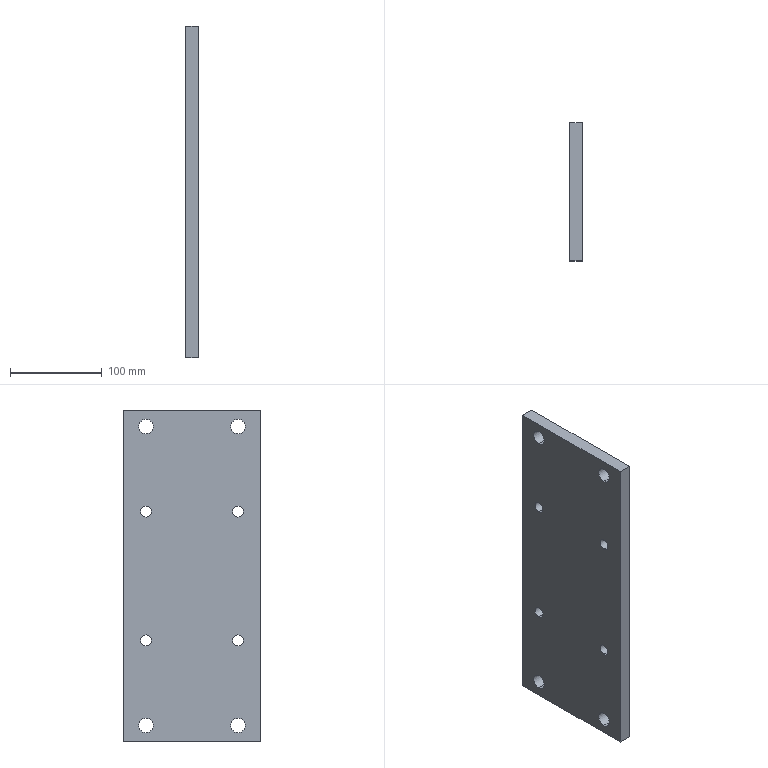Part | SolidWorks | features BaseBody 1 | 1 solid | 22 faces | box 14 x 150 x 360 mm | volume 738407 mm3 | cylinder 16 | plane 6 | commonest cylinder face diameters 12 x8 16 x8
STEP:
#1=CARTESIAN_POINT('',(14.,50.,-76.));
#2=VERTEX_POINT('',#1);
#3=CARTESIAN_POINT('',(14.,50.,-64.));
#4=VERTEX_POINT('',#3);
#5=CARTESIAN_POINT('',(14.,50.,-70.));
#6=DIRECTION('',(-1.,0.,0.));
#7=DIRECTION('',(0.,0.,1.));
#8=AXIS2_PLACEMENT_3D('',#5,#6,#7);
#9=CIRCLE('',#8,6.);
#10=EDGE_CURVE('',#2,#4,#9,.T.);
#11=ORIENTED_EDGE('',*,*,#10,.F.);
#12=CARTESIAN_POINT('',(0.,50.,-76.));
#13=VERTEX_POINT('',#12);
#14=CARTESIAN_POINT('',(14.,50.,-76.));
#15=DIRECTION('',(-1.,0.,0.));
#16=VECTOR('',#15,1000.);
#17=LINE('',#14,#16);
#18=EDGE_CURVE('',#2,#13,#17,.T.);
#19=ORIENTED_EDGE('',*,*,#18,.T.);
#20=CARTESIAN_POINT('',(0.,50.,-64.));
#21=VERTEX_POINT('',#20);
#22=CARTESIAN_POINT('',(0.,50.,-70.));
#23=DIRECTION('',(1.,0.,0.));
#24=DIRECTION('',(0.,0.,1.));
#25=AXIS2_PLACEMENT_3D('',#22,#23,#24);
#26=CIRCLE('',#25,6.);
#27=EDGE_CURVE('',#21,#13,#26,.T.);
#28=ORIENTED_EDGE('',*,*,#27,.F.);
#29=CARTESIAN_POINT('',(14.,50.,-64.));
#30=DIRECTION('',(-1.,0.,0.));
#31=VECTOR('',#30,1000.);
#32=LINE('',#29,#31);
#33=EDGE_CURVE('',#4,#21,#32,.T.);
#34=ORIENTED_EDGE('',*,*,#33,.F.);
#35=EDGE_LOOP('',(#11,#19,#28,#34));
#36=FACE_OUTER_BOUND('',#35,.T.);
#37=CARTESIAN_POINT('',(14.,50.,-70.));
#38=DIRECTION('',(-1.,0.,0.));
#39=DIRECTION('',(0.,0.,1.));
#40=AXIS2_PLACEMENT_3D('',#37,#38,#39);
#41=CYLINDRICAL_SURFACE('',#40,6.);
#42=ADVANCED_FACE('',(#36),#41,.F.);
#43=CARTESIAN_POINT('',(14.,-50.,64.));
#44=VERTEX_POINT('',#43);
#45=CARTESIAN_POINT('',(14.,-50.,76.));
#46=VERTEX_POINT('',#45);
#47=CARTESIAN_POINT('',(14.,-50.,70.));
#48=DIRECTION('',(-1.,0.,0.));
#49=DIRECTION('',(0.,0.,1.));
#50=AXIS2_PLACEMENT_3D('',#47,#48,#49);
#51=CIRCLE('',#50,6.);
#52=EDGE_CURVE('',#44,#46,#51,.T.);
#53=ORIENTED_EDGE('',*,*,#52,.F.);
#54=CARTESIAN_POINT('',(0.,-50.,64.));
#55=VERTEX_POINT('',#54);
#56=CARTESIAN_POINT('',(14.,-50.,64.));
#57=DIRECTION('',(-1.,0.,0.));
#58=VECTOR('',#57,1000.);
#59=LINE('',#56,#58);
#60=EDGE_CURVE('',#44,#55,#59,.T.);
#61=ORIENTED_EDGE('',*,*,#60,.T.);
#62=CARTESIAN_POINT('',(0.,-50.,76.));
#63=VERTEX_POINT('',#62);
#64=CARTESIAN_POINT('',(0.,-50.,70.));
#65=DIRECTION('',(1.,0.,0.));
#66=DIRECTION('',(0.,0.,1.));
#67=AXIS2_PLACEMENT_3D('',#64,#65,#66);
#68=CIRCLE('',#67,6.);
#69=EDGE_CURVE('',#63,#55,#68,.T.);
#70=ORIENTED_EDGE('',*,*,#69,.F.);
#71=CARTESIAN_POINT('',(14.,-50.,76.));
#72=DIRECTION('',(-1.,0.,0.));
#73=VECTOR('',#72,1000.);
#74=LINE('',#71,#73);
#75=EDGE_CURVE('',#46,#63,#74,.T.);
#76=ORIENTED_EDGE('',*,*,#75,.F.);
#77=EDGE_LOOP('',(#53,#61,#70,#76));
#78=FACE_OUTER_BOUND('',#77,.T.);
#79=CARTESIAN_POINT('',(14.,-50.,70.));
#80=DIRECTION('',(-1.,0.,0.));
#81=DIRECTION('',(0.,0.,1.));
#82=AXIS2_PLACEMENT_3D('',#79,#80,#81);
#83=CYLINDRICAL_SURFACE('',#82,6.);
#84=ADVANCED_FACE('',(#78),#83,.F.);
#85=CARTESIAN_POINT('',(14.,50.,64.));
#86=VERTEX_POINT('',#85);
#87=CARTESIAN_POINT('',(14.,50.,76.));
#88=VERTEX_POINT('',#87);
#89=CARTESIAN_POINT('',(14.,50.,70.));
#90=DIRECTION('',(-1.,0.,0.));
#91=DIRECTION('',(0.,0.,1.));
#92=AXIS2_PLACEMENT_3D('',#89,#90,#91);
#93=CIRCLE('',#92,6.);
#94=EDGE_CURVE('',#86,#88,#93,.T.);
#95=ORIENTED_EDGE('',*,*,#94,.F.);
#96=CARTESIAN_POINT('',(0.,50.,64.));
#97=VERTEX_POINT('',#96);
#98=CARTESIAN_POINT('',(14.,50.,64.));
#99=DIRECTION('',(-1.,0.,0.));
#100=VECTOR('',#99,1000.);
#101=LINE('',#98,#100);
#102=EDGE_CURVE('',#86,#97,#101,.T.);
#103=ORIENTED_EDGE('',*,*,#102,.T.);
#104=CARTESIAN_POINT('',(0.,50.,76.));
#105=VERTEX_POINT('',#104);
#106=CARTESIAN_POINT('',(0.,50.,70.));
#107=DIRECTION('',(1.,0.,0.));
#108=DIRECTION('',(0.,0.,1.));
#109=AXIS2_PLACEMENT_3D('',#106,#107,#108);
#110=CIRCLE('',#109,6.);
#111=EDGE_CURVE('',#105,#97,#110,.T.);
#112=ORIENTED_EDGE('',*,*,#111,.F.);
#113=CARTESIAN_POINT('',(14.,50.,76.));
#114=DIRECTION('',(-1.,0.,0.));
#115=VECTOR('',#114,1000.);
#116=LINE('',#113,#115);
#117=EDGE_CURVE('',#88,#105,#116,.T.);
#118=ORIENTED_EDGE('',*,*,#117,.F.);
#119=EDGE_LOOP('',(#95,#103,#112,#118));
#120=FACE_OUTER_BOUND('',#119,.T.);
#121=CARTESIAN_POINT('',(14.,50.,70.));
#122=DIRECTION('',(-1.,0.,0.));
#123=DIRECTION('',(0.,0.,1.));
#124=AXIS2_PLACEMENT_3D('',#121,#122,#123);
#125=CYLINDRICAL_SURFACE('',#124,6.);
#126=ADVANCED_FACE('',(#120),#125,.F.);
#127=CARTESIAN_POINT('',(14.,-50.,-76.));
#128=VERTEX_POINT('',#127);
#129=CARTESIAN_POINT('',(14.,-50.,-64.));
#130=VERTEX_POINT('',#129);
#131=CARTESIAN_POINT('',(14.,-50.,-70.));
#132=DIRECTION('',(-1.,0.,0.));
#133=DIRECTION('',(0.,0.,1.));
#134=AXIS2_PLACEMENT_3D('',#131,#132,#133);
#135=CIRCLE('',#134,6.);
#136=EDGE_CURVE('',#128,#130,#135,.T.);
#137=ORIENTED_EDGE('',*,*,#136,.F.);
#138=CARTESIAN_POINT('',(0.,-50.,-76.));
#139=VERTEX_POINT('',#138);
#140=CARTESIAN_POINT('',(14.,-50.,-76.));
#141=DIRECTION('',(-1.,0.,0.));
#142=VECTOR('',#141,1000.);
#143=LINE('',#140,#142);
#144=EDGE_CURVE('',#128,#139,#143,.T.);
#145=ORIENTED_EDGE('',*,*,#144,.T.);
#146=CARTESIAN_POINT('',(0.,-50.,-64.));
#147=VERTEX_POINT('',#146);
#148=CARTESIAN_POINT('',(0.,-50.,-70.));
#149=DIRECTION('',(1.,0.,0.));
#150=DIRECTION('',(0.,0.,1.));
#151=AXIS2_PLACEMENT_3D('',#148,#149,#150);
#152=CIRCLE('',#151,6.);
#153=EDGE_CURVE('',#147,#139,#152,.T.);
#154=ORIENTED_EDGE('',*,*,#153,.F.);
#155=CARTESIAN_POINT('',(14.,-50.,-64.));
#156=DIRECTION('',(-1.,0.,0.));
#157=VECTOR('',#156,1000.);
#158=LINE('',#155,#157);
#159=EDGE_CURVE('',#130,#147,#158,.T.);
#160=ORIENTED_EDGE('',*,*,#159,.F.);
#161=EDGE_LOOP('',(#137,#145,#154,#160));
#162=FACE_OUTER_BOUND('',#161,.T.);
#163=CARTESIAN_POINT('',(14.,-50.,-70.));
#164=DIRECTION('',(-1.,0.,0.));
#165=DIRECTION('',(0.,0.,1.));
#166=AXIS2_PLACEMENT_3D('',#163,#164,#165);
#167=CYLINDRICAL_SURFACE('',#166,6.);
#168=ADVANCED_FACE('',(#162),#167,.F.);
#169=CARTESIAN_POINT('',(14.,50.,-170.5));
#170=VERTEX_POINT('',#169);
#171=CARTESIAN_POINT('',(14.,50.,-154.5));
#172=VERTEX_POINT('',#171);
#173=CARTESIAN_POINT('',(14.,50.,-162.5));
#174=DIRECTION('',(-1.,0.,0.));
#175=DIRECTION('',(0.,0.,1.));
#176=AXIS2_PLACEMENT_3D('',#173,#174,#175);
#177=CIRCLE('',#176,8.);
#178=EDGE_CURVE('',#170,#172,#177,.T.);
#179=ORIENTED_EDGE('',*,*,#178,.F.);
#180=CARTESIAN_POINT('',(0.,50.,-170.5));
#181=VERTEX_POINT('',#180);
#182=CARTESIAN_POINT('',(14.,50.,-170.5));
#183=DIRECTION('',(-1.,0.,0.));
#184=VECTOR('',#183,1000.);
#185=LINE('',#182,#184);
#186=EDGE_CURVE('',#170,#181,#185,.T.);
#187=ORIENTED_EDGE('',*,*,#186,.T.);
#188=CARTESIAN_POINT('',(0.,50.,-154.5));
#189=VERTEX_POINT('',#188);
#190=CARTESIAN_POINT('',(0.,50.,-162.5));
#191=DIRECTION('',(1.,0.,0.));
#192=DIRECTION('',(0.,0.,1.));
#193=AXIS2_PLACEMENT_3D('',#190,#191,#192);
#194=CIRCLE('',#193,8.);
#195=EDGE_CURVE('',#189,#181,#194,.T.);
#196=ORIENTED_EDGE('',*,*,#195,.F.);
#197=CARTESIAN_POINT('',(14.,50.,-154.5));
#198=DIRECTION('',(-1.,0.,0.));
#199=VECTOR('',#198,1000.);
#200=LINE('',#197,#199);
#201=EDGE_CURVE('',#172,#189,#200,.T.);
#202=ORIENTED_EDGE('',*,*,#201,.F.);
#203=EDGE_LOOP('',(#179,#187,#196,#202));
#204=FACE_OUTER_BOUND('',#203,.T.);
#205=CARTESIAN_POINT('',(14.,50.,-162.5));
#206=DIRECTION('',(-1.,0.,0.));
#207=DIRECTION('',(0.,0.,1.));
#208=AXIS2_PLACEMENT_3D('',#205,#206,#207);
#209=CYLINDRICAL_SURFACE('',#208,8.);
#210=ADVANCED_FACE('',(#204),#209,.F.);
#211=CARTESIAN_POINT('',(14.,-50.,-170.5));
#212=VERTEX_POINT('',#211);
#213=CARTESIAN_POINT('',(14.,-50.,-154.5));
#214=VERTEX_POINT('',#213);
#215=CARTESIAN_POINT('',(14.,-50.,-162.5));
#216=DIRECTION('',(-1.,0.,0.));
#217=DIRECTION('',(0.,0.,1.));
#218=AXIS2_PLACEMENT_3D('',#215,#216,#217);
#219=CIRCLE('',#218,8.);
#220=EDGE_CURVE('',#212,#214,#219,.T.);
#221=ORIENTED_EDGE('',*,*,#220,.F.);
#222=CARTESIAN_POINT('',(0.,-50.,-170.5));
#223=VERTEX_POINT('',#222);
#224=CARTESIAN_POINT('',(14.,-50.,-170.5));
#225=DIRECTION('',(-1.,0.,0.));
#226=VECTOR('',#225,1000.);
#227=LINE('',#224,#226);
#228=EDGE_CURVE('',#212,#223,#227,.T.);
#229=ORIENTED_EDGE('',*,*,#228,.T.);
#230=CARTESIAN_POINT('',(0.,-50.,-154.5));
#231=VERTEX_POINT('',#230);
#232=CARTESIAN_POINT('',(0.,-50.,-162.5));
#233=DIRECTION('',(1.,0.,0.));
#234=DIRECTION('',(0.,0.,1.));
#235=AXIS2_PLACEMENT_3D('',#232,#233,#234);
#236=CIRCLE('',#235,8.);
#237=EDGE_CURVE('',#231,#223,#236,.T.);
#238=ORIENTED_EDGE('',*,*,#237,.F.);
#239=CARTESIAN_POINT('',(14.,-50.,-154.5));
#240=DIRECTION('',(-1.,0.,0.));
#241=VECTOR('',#240,1000.);
#242=LINE('',#239,#241);
#243=EDGE_CURVE('',#214,#231,#242,.T.);
#244=ORIENTED_EDGE('',*,*,#243,.F.);
#245=EDGE_LOOP('',(#221,#229,#238,#244));
#246=FACE_OUTER_BOUND('',#245,.T.);
#247=CARTESIAN_POINT('',(14.,-50.,-162.5));
#248=DIRECTION('',(-1.,0.,0.));
#249=DIRECTION('',(0.,0.,1.));
#250=AXIS2_PLACEMENT_3D('',#247,#248,#249);
#251=CYLINDRICAL_SURFACE('',#250,8.);
#252=ADVANCED_FACE('',(#246),#251,.F.);
#253=CARTESIAN_POINT('',(14.,-50.,154.5));
#254=VERTEX_POINT('',#253);
#255=CARTESIAN_POINT('',(14.,-50.,170.5));
#256=VERTEX_POINT('',#255);
#257=CARTESIAN_POINT('',(14.,-50.,162.5));
#258=DIRECTION('',(-1.,0.,0.));
#259=DIRECTION('',(0.,0.,1.));
#260=AXIS2_PLACEMENT_3D('',#257,#258,#259);
#261=CIRCLE('',#260,8.);
#262=EDGE_CURVE('',#254,#256,#261,.T.);
#263=ORIENTED_EDGE('',*,*,#262,.F.);
#264=CARTESIAN_POINT('',(0.,-50.,154.5));
#265=VERTEX_POINT('',#264);
#266=CARTESIAN_POINT('',(14.,-50.,154.5));
#267=DIRECTION('',(-1.,0.,0.));
#268=VECTOR('',#267,1000.);
#269=LINE('',#266,#268);
#270=EDGE_CURVE('',#254,#265,#269,.T.);
#271=ORIENTED_EDGE('',*,*,#270,.T.);
#272=CARTESIAN_POINT('',(0.,-50.,170.5));
#273=VERTEX_POINT('',#272);
#274=CARTESIAN_POINT('',(0.,-50.,162.5));
#275=DIRECTION('',(1.,0.,0.));
#276=DIRECTION('',(0.,0.,1.));
#277=AXIS2_PLACEMENT_3D('',#274,#275,#276);
#278=CIRCLE('',#277,8.);
#279=EDGE_CURVE('',#273,#265,#278,.T.);
#280=ORIENTED_EDGE('',*,*,#279,.F.);
#281=CARTESIAN_POINT('',(14.,-50.,170.5));
#282=DIRECTION('',(-1.,0.,0.));
#283=VECTOR('',#282,1000.);
#284=LINE('',#281,#283);
#285=EDGE_CURVE('',#256,#273,#284,.T.);
#286=ORIENTED_EDGE('',*,*,#285,.F.);
#287=EDGE_LOOP('',(#263,#271,#280,#286));
#288=FACE_OUTER_BOUND('',#287,.T.);
#289=CARTESIAN_POINT('',(14.,-50.,162.5));
#290=DIRECTION('',(-1.,0.,0.));
#291=DIRECTION('',(0.,0.,1.));
#292=AXIS2_PLACEMENT_3D('',#289,#290,#291);
#293=CYLINDRICAL_SURFACE('',#292,8.);
#294=ADVANCED_FACE('',(#288),#293,.F.);
#295=CARTESIAN_POINT('',(14.,50.,154.5));
#296=VERTEX_POINT('',#295);
#297=CARTESIAN_POINT('',(14.,50.,170.5));
#298=VERTEX_POINT('',#297);
#299=CARTESIAN_POINT('',(14.,50.,162.5));
#300=DIRECTION('',(-1.,0.,0.));
#301=DIRECTION('',(0.,0.,1.));
#302=AXIS2_PLACEMENT_3D('',#299,#300,#301);
#303=CIRCLE('',#302,8.);
#304=EDGE_CURVE('',#296,#298,#303,.T.);
#305=ORIENTED_EDGE('',*,*,#304,.F.);
#306=CARTESIAN_POINT('',(0.,50.,154.5));
#307=VERTEX_POINT('',#306);
#308=CARTESIAN_POINT('',(14.,50.,154.5));
#309=DIRECTION('',(-1.,0.,0.));
#310=VECTOR('',#309,1000.);
#311=LINE('',#308,#310);
#312=EDGE_CURVE('',#296,#307,#311,.T.);
#313=ORIENTED_EDGE('',*,*,#312,.T.);
#314=CARTESIAN_POINT('',(0.,50.,170.5));
#315=VERTEX_POINT('',#314);
#316=CARTESIAN_POINT('',(0.,50.,162.5));
#317=DIRECTION('',(1.,0.,0.));
#318=DIRECTION('',(0.,0.,1.));
#319=AXIS2_PLACEMENT_3D('',#316,#317,#318);
#320=CIRCLE('',#319,8.);
#321=EDGE_CURVE('',#315,#307,#320,.T.);
#322=ORIENTED_EDGE('',*,*,#321,.F.);
#323=CARTESIAN_POINT('',(14.,50.,170.5));
#324=DIRECTION('',(-1.,0.,0.));
#325=VECTOR('',#324,1000.);
#326=LINE('',#323,#325);
#327=EDGE_CURVE('',#298,#315,#326,.T.);
#328=ORIENTED_EDGE('',*,*,#327,.F.);
#329=EDGE_LOOP('',(#305,#313,#322,#328));
#330=FACE_OUTER_BOUND('',#329,.T.);
#331=CARTESIAN_POINT('',(14.,50.,162.5));
#332=DIRECTION('',(-1.,0.,0.));
#333=DIRECTION('',(0.,0.,1.));
#334=AXIS2_PLACEMENT_3D('',#331,#332,#333);
#335=CYLINDRICAL_SURFACE('',#334,8.);
#336=ADVANCED_FACE('',(#330),#335,.F.);
#337=ORIENTED_EDGE('',*,*,#27,.T.);
#338=CARTESIAN_POINT('',(0.,50.,-70.));
#339=DIRECTION('',(1.,0.,0.));
#340=DIRECTION('',(0.,0.,1.));
#341=AXIS2_PLACEMENT_3D('',#338,#339,#340);
#342=CIRCLE('',#341,6.);
#343=EDGE_CURVE('',#13,#21,#342,.T.);
#344=ORIENTED_EDGE('',*,*,#343,.T.);
#345=EDGE_LOOP('',(#337,#344));
#346=FACE_BOUND('',#345,.T.);
#347=ORIENTED_EDGE('',*,*,#69,.T.);
#348=CARTESIAN_POINT('',(0.,-50.,70.));
#349=DIRECTION('',(1.,0.,0.));
#350=DIRECTION('',(0.,0.,1.));
#351=AXIS2_PLACEMENT_3D('',#348,#349,#350);
#352=CIRCLE('',#351,6.);
#353=EDGE_CURVE('',#55,#63,#352,.T.);
#354=ORIENTED_EDGE('',*,*,#353,.T.);
#355=EDGE_LOOP('',(#347,#354));
#356=FACE_BOUND('',#355,.T.);
#357=CARTESIAN_POINT('',(0.,-75.,180.));
#358=VERTEX_POINT('',#357);
#359=CARTESIAN_POINT('',(0.,75.,180.));
#360=VERTEX_POINT('',#359);
#361=CARTESIAN_POINT('',(0.,0.,180.));
#362=DIRECTION('',(0.,1.,0.));
#363=VECTOR('',#362,1000.);
#364=LINE('',#361,#363);
#365=EDGE_CURVE('',#358,#360,#364,.T.);
#366=ORIENTED_EDGE('',*,*,#365,.T.);
#367=CARTESIAN_POINT('',(0.,75.,-180.));
#368=VERTEX_POINT('',#367);
#369=CARTESIAN_POINT('',(0.,75.,0.));
#370=DIRECTION('',(0.,0.,-1.));
#371=VECTOR('',#370,1000.);
#372=LINE('',#369,#371);
#373=EDGE_CURVE('',#360,#368,#372,.T.);
#374=ORIENTED_EDGE('',*,*,#373,.T.);
#375=CARTESIAN_POINT('',(0.,-75.,-180.));
#376=VERTEX_POINT('',#375);
#377=CARTESIAN_POINT('',(0.,0.,-180.));
#378=DIRECTION('',(0.,-1.,0.));
#379=VECTOR('',#378,1000.);
#380=LINE('',#377,#379);
#381=EDGE_CURVE('',#368,#376,#380,.T.);
#382=ORIENTED_EDGE('',*,*,#381,.T.);
#383=CARTESIAN_POINT('',(0.,-75.,0.));
#384=DIRECTION('',(0.,0.,1.));
#385=VECTOR('',#384,1000.);
#386=LINE('',#383,#385);
#387=EDGE_CURVE('',#376,#358,#386,.T.);
#388=ORIENTED_EDGE('',*,*,#387,.T.);
#389=EDGE_LOOP('',(#366,#374,#382,#388));
#390=FACE_OUTER_BOUND('',#389,.T.);
#391=ORIENTED_EDGE('',*,*,#111,.T.);
#392=CARTESIAN_POINT('',(0.,50.,70.));
#393=DIRECTION('',(1.,0.,0.));
#394=DIRECTION('',(0.,0.,1.));
#395=AXIS2_PLACEMENT_3D('',#392,#393,#394);
#396=CIRCLE('',#395,6.);
#397=EDGE_CURVE('',#97,#105,#396,.T.);
#398=ORIENTED_EDGE('',*,*,#397,.T.);
#399=EDGE_LOOP('',(#391,#398));
#400=FACE_BOUND('',#399,.T.);
#401=ORIENTED_EDGE('',*,*,#153,.T.);
#402=CARTESIAN_POINT('',(0.,-50.,-70.));
#403=DIRECTION('',(1.,0.,0.));
#404=DIRECTION('',(0.,0.,1.));
#405=AXIS2_PLACEMENT_3D('',#402,#403,#404);
#406=CIRCLE('',#405,6.);
#407=EDGE_CURVE('',#139,#147,#406,.T.);
#408=ORIENTED_EDGE('',*,*,#407,.T.);
#409=EDGE_LOOP('',(#401,#408));
#410=FACE_BOUND('',#409,.T.);
#411=ORIENTED_EDGE('',*,*,#195,.T.);
#412=CARTESIAN_POINT('',(0.,50.,-162.5));
#413=DIRECTION('',(1.,0.,0.));
#414=DIRECTION('',(0.,0.,1.));
#415=AXIS2_PLACEMENT_3D('',#412,#413,#414);
#416=CIRCLE('',#415,8.);
#417=EDGE_CURVE('',#181,#189,#416,.T.);
#418=ORIENTED_EDGE('',*,*,#417,.T.);
#419=EDGE_LOOP('',(#411,#418));
#420=FACE_BOUND('',#419,.T.);
#421=ORIENTED_EDGE('',*,*,#237,.T.);
#422=CARTESIAN_POINT('',(0.,-50.,-162.5));
#423=DIRECTION('',(1.,0.,0.));
#424=DIRECTION('',(0.,0.,1.));
#425=AXIS2_PLACEMENT_3D('',#422,#423,#424);
#426=CIRCLE('',#425,8.);
#427=EDGE_CURVE('',#223,#231,#426,.T.);
#428=ORIENTED_EDGE('',*,*,#427,.T.);
#429=EDGE_LOOP('',(#421,#428));
#430=FACE_BOUND('',#429,.T.);
#431=ORIENTED_EDGE('',*,*,#279,.T.);
#432=CARTESIAN_POINT('',(0.,-50.,162.5));
#433=DIRECTION('',(1.,0.,0.));
#434=DIRECTION('',(0.,0.,1.));
#435=AXIS2_PLACEMENT_3D('',#432,#433,#434);
#436=CIRCLE('',#435,8.);
#437=EDGE_CURVE('',#265,#273,#436,.T.);
#438=ORIENTED_EDGE('',*,*,#437,.T.);
#439=EDGE_LOOP('',(#431,#438));
#440=FACE_BOUND('',#439,.T.);
#441=ORIENTED_EDGE('',*,*,#321,.T.);
#442=CARTESIAN_POINT('',(0.,50.,162.5));
#443=DIRECTION('',(1.,0.,0.));
#444=DIRECTION('',(0.,0.,1.));
#445=AXIS2_PLACEMENT_3D('',#442,#443,#444);
#446=CIRCLE('',#445,8.);
#447=EDGE_CURVE('',#307,#315,#446,.T.);
#448=ORIENTED_EDGE('',*,*,#447,.T.);
#449=EDGE_LOOP('',(#441,#448));
#450=FACE_BOUND('',#449,.T.);
#451=CARTESIAN_POINT('',(0.,0.,0.));
#452=DIRECTION('',(-1.,0.,0.));
#453=DIRECTION('',(0.,0.,1.));
#454=AXIS2_PLACEMENT_3D('',#451,#452,#453);
#455=PLANE('',#454);
#456=ADVANCED_FACE('',(#346,#356,#390,#400,#410,#420,#430,#440,#450),#455,.T.);
#457=ORIENTED_EDGE('',*,*,#18,.F.);
#458=CARTESIAN_POINT('',(14.,50.,-70.));
#459=DIRECTION('',(-1.,0.,0.));
#460=DIRECTION('',(0.,0.,1.));
#461=AXIS2_PLACEMENT_3D('',#458,#459,#460);
#462=CIRCLE('',#461,6.);
#463=EDGE_CURVE('',#4,#2,#462,.T.);
#464=ORIENTED_EDGE('',*,*,#463,.F.);
#465=ORIENTED_EDGE('',*,*,#33,.T.);
#466=ORIENTED_EDGE('',*,*,#343,.F.);
#467=EDGE_LOOP('',(#457,#464,#465,#466));
#468=FACE_OUTER_BOUND('',#467,.T.);
#469=CARTESIAN_POINT('',(14.,50.,-70.));
#470=DIRECTION('',(-1.,0.,0.));
#471=DIRECTION('',(0.,0.,1.));
#472=AXIS2_PLACEMENT_3D('',#469,#470,#471);
#473=CYLINDRICAL_SURFACE('',#472,6.);
#474=ADVANCED_FACE('',(#468),#473,.F.);
#475=ORIENTED_EDGE('',*,*,#60,.F.);
#476=CARTESIAN_POINT('',(14.,-50.,70.));
#477=DIRECTION('',(-1.,0.,0.));
#478=DIRECTION('',(0.,0.,1.));
#479=AXIS2_PLACEMENT_3D('',#476,#477,#478);
#480=CIRCLE('',#479,6.);
#481=EDGE_CURVE('',#46,#44,#480,.T.);
#482=ORIENTED_EDGE('',*,*,#481,.F.);
#483=ORIENTED_EDGE('',*,*,#75,.T.);
#484=ORIENTED_EDGE('',*,*,#353,.F.);
#485=EDGE_LOOP('',(#475,#482,#483,#484));
#486=FACE_OUTER_BOUND('',#485,.T.);
#487=CARTESIAN_POINT('',(14.,-50.,70.));
#488=DIRECTION('',(-1.,0.,0.));
#489=DIRECTION('',(0.,0.,1.));
#490=AXIS2_PLACEMENT_3D('',#487,#488,#489);
#491=CYLINDRICAL_SURFACE('',#490,6.);
#492=ADVANCED_FACE('',(#486),#491,.F.);
#493=CARTESIAN_POINT('',(14.,75.,180.));
#494=VERTEX_POINT('',#493);
#495=CARTESIAN_POINT('',(14.,75.,180.));
#496=DIRECTION('',(-1.,0.,0.));
#497=VECTOR('',#496,1000.);
#498=LINE('',#495,#497);
#499=EDGE_CURVE('',#494,#360,#498,.T.);
#500=ORIENTED_EDGE('',*,*,#499,.F.);
#501=CARTESIAN_POINT('',(14.,75.,-180.));
#502=VERTEX_POINT('',#501);
#503=CARTESIAN_POINT('',(14.,75.,180.));
#504=DIRECTION('',(0.,0.,1.));
#505=VECTOR('',#504,1000.);
#506=LINE('',#503,#505);
#507=EDGE_CURVE('',#502,#494,#506,.T.);
#508=ORIENTED_EDGE('',*,*,#507,.F.);
#509=CARTESIAN_POINT('',(14.,75.,-180.));
#510=DIRECTION('',(1.,0.,0.));
#511=VECTOR('',#510,1000.);
#512=LINE('',#509,#511);
#513=EDGE_CURVE('',#368,#502,#512,.T.);
#514=ORIENTED_EDGE('',*,*,#513,.F.);
#515=ORIENTED_EDGE('',*,*,#373,.F.);
#516=EDGE_LOOP('',(#500,#508,#514,#515));
#517=FACE_OUTER_BOUND('',#516,.T.);
#518=CARTESIAN_POINT('',(14.,75.,180.));
#519=DIRECTION('',(0.,-1.,0.));
#520=DIRECTION('',(0.,0.,-1.));
#521=AXIS2_PLACEMENT_3D('',#518,#519,#520);
#522=PLANE('',#521);
#523=ADVANCED_FACE('',(#517),#522,.F.);
#524=CARTESIAN_POINT('',(14.,-75.,180.));
#525=VERTEX_POINT('',#524);
#526=CARTESIAN_POINT('',(14.,-75.,180.));
#527=DIRECTION('',(-1.,0.,0.));
#528=VECTOR('',#527,1000.);
#529=LINE('',#526,#528);
#530=EDGE_CURVE('',#525,#358,#529,.T.);
#531=ORIENTED_EDGE('',*,*,#530,.F.);
#532=CARTESIAN_POINT('',(14.,-75.,180.));
#533=DIRECTION('',(0.,-1.,0.));
#534=VECTOR('',#533,1000.);
#535=LINE('',#532,#534);
#536=EDGE_CURVE('',#494,#525,#535,.T.);
#537=ORIENTED_EDGE('',*,*,#536,.F.);
#538=ORIENTED_EDGE('',*,*,#499,.T.);
#539=ORIENTED_EDGE('',*,*,#365,.F.);
#540=EDGE_LOOP('',(#531,#537,#538,#539));
#541=FACE_OUTER_BOUND('',#540,.T.);
#542=CARTESIAN_POINT('',(14.,-75.,180.));
#543=DIRECTION('',(0.,0.,-1.));
#544=DIRECTION('',(-1.,0.,0.));
#545=AXIS2_PLACEMENT_3D('',#542,#543,#544);
#546=PLANE('',#545);
#547=ADVANCED_FACE('',(#541),#546,.F.);
#548=CARTESIAN_POINT('',(14.,-75.,-180.));
#549=VERTEX_POINT('',#548);
#550=CARTESIAN_POINT('',(14.,-75.,-180.));
#551=DIRECTION('',(-1.,0.,0.));
#552=VECTOR('',#551,1000.);
#553=LINE('',#550,#552);
#554=EDGE_CURVE('',#549,#376,#553,.T.);
#555=ORIENTED_EDGE('',*,*,#554,.F.);
#556=CARTESIAN_POINT('',(14.,-75.,180.));
#557=DIRECTION('',(0.,0.,-1.));
#558=VECTOR('',#557,1000.);
#559=LINE('',#556,#558);
#560=EDGE_CURVE('',#525,#549,#559,.T.);
#561=ORIENTED_EDGE('',*,*,#560,.F.);
#562=ORIENTED_EDGE('',*,*,#530,.T.);
#563=ORIENTED_EDGE('',*,*,#387,.F.);
#564=EDGE_LOOP('',(#555,#561,#562,#563));
#565=FACE_OUTER_BOUND('',#564,.T.);
#566=CARTESIAN_POINT('',(14.,-75.,180.));
#567=DIRECTION('',(0.,1.,0.));
#568=DIRECTION('',(0.,0.,1.));
#569=AXIS2_PLACEMENT_3D('',#566,#567,#568);
#570=PLANE('',#569);
#571=ADVANCED_FACE('',(#565),#570,.F.);
#572=ORIENTED_EDGE('',*,*,#513,.T.);
#573=CARTESIAN_POINT('',(14.,-75.,-180.));
#574=DIRECTION('',(0.,1.,0.));
#575=VECTOR('',#574,1000.);
#576=LINE('',#573,#575);
#577=EDGE_CURVE('',#549,#502,#576,.T.);
#578=ORIENTED_EDGE('',*,*,#577,.F.);
#579=ORIENTED_EDGE('',*,*,#554,.T.);
#580=ORIENTED_EDGE('',*,*,#381,.F.);
#581=EDGE_LOOP('',(#572,#578,#579,#580));
#582=FACE_OUTER_BOUND('',#581,.T.);
#583=CARTESIAN_POINT('',(14.,-75.,-180.));
#584=DIRECTION('',(0.,0.,1.));
#585=DIRECTION('',(1.,0.,0.));
#586=AXIS2_PLACEMENT_3D('',#583,#584,#585);
#587=PLANE('',#586);
#588=ADVANCED_FACE('',(#582),#587,.F.);
#589=ORIENTED_EDGE('',*,*,#102,.F.);
#590=CARTESIAN_POINT('',(14.,50.,70.));
#591=DIRECTION('',(-1.,0.,0.));
#592=DIRECTION('',(0.,0.,1.));
#593=AXIS2_PLACEMENT_3D('',#590,#591,#592);
#594=CIRCLE('',#593,6.);
#595=EDGE_CURVE('',#88,#86,#594,.T.);
#596=ORIENTED_EDGE('',*,*,#595,.F.);
#597=ORIENTED_EDGE('',*,*,#117,.T.);
#598=ORIENTED_EDGE('',*,*,#397,.F.);
#599=EDGE_LOOP('',(#589,#596,#597,#598));
#600=FACE_OUTER_BOUND('',#599,.T.);
#601=CARTESIAN_POINT('',(14.,50.,70.));
#602=DIRECTION('',(-1.,0.,0.));
#603=DIRECTION('',(0.,0.,1.));
#604=AXIS2_PLACEMENT_3D('',#601,#602,#603);
#605=CYLINDRICAL_SURFACE('',#604,6.);
#606=ADVANCED_FACE('',(#600),#605,.F.);
#607=ORIENTED_EDGE('',*,*,#144,.F.);
#608=CARTESIAN_POINT('',(14.,-50.,-70.));
#609=DIRECTION('',(-1.,0.,0.));
#610=DIRECTION('',(0.,0.,1.));
#611=AXIS2_PLACEMENT_3D('',#608,#609,#610);
#612=CIRCLE('',#611,6.);
#613=EDGE_CURVE('',#130,#128,#612,.T.);
#614=ORIENTED_EDGE('',*,*,#613,.F.);
#615=ORIENTED_EDGE('',*,*,#159,.T.);
#616=ORIENTED_EDGE('',*,*,#407,.F.);
#617=EDGE_LOOP('',(#607,#614,#615,#616));
#618=FACE_OUTER_BOUND('',#617,.T.);
#619=CARTESIAN_POINT('',(14.,-50.,-70.));
#620=DIRECTION('',(-1.,0.,0.));
#621=DIRECTION('',(0.,0.,1.));
#622=AXIS2_PLACEMENT_3D('',#619,#620,#621);
#623=CYLINDRICAL_SURFACE('',#622,6.);
#624=ADVANCED_FACE('',(#618),#623,.F.);
#625=ORIENTED_EDGE('',*,*,#186,.F.);
#626=CARTESIAN_POINT('',(14.,50.,-162.5));
#627=DIRECTION('',(-1.,0.,0.));
#628=DIRECTION('',(0.,0.,1.));
#629=AXIS2_PLACEMENT_3D('',#626,#627,#628);
#630=CIRCLE('',#629,8.);
#631=EDGE_CURVE('',#172,#170,#630,.T.);
#632=ORIENTED_EDGE('',*,*,#631,.F.);
#633=ORIENTED_EDGE('',*,*,#201,.T.);
#634=ORIENTED_EDGE('',*,*,#417,.F.);
#635=EDGE_LOOP('',(#625,#632,#633,#634));
#636=FACE_OUTER_BOUND('',#635,.T.);
#637=CARTESIAN_POINT('',(14.,50.,-162.5));
#638=DIRECTION('',(-1.,0.,0.));
#639=DIRECTION('',(0.,0.,1.));
#640=AXIS2_PLACEMENT_3D('',#637,#638,#639);
#641=CYLINDRICAL_SURFACE('',#640,8.);
#642=ADVANCED_FACE('',(#636),#641,.F.);
#643=ORIENTED_EDGE('',*,*,#228,.F.);
#644=CARTESIAN_POINT('',(14.,-50.,-162.5));
#645=DIRECTION('',(-1.,0.,0.));
#646=DIRECTION('',(0.,0.,1.));
#647=AXIS2_PLACEMENT_3D('',#644,#645,#646);
#648=CIRCLE('',#647,8.);
#649=EDGE_CURVE('',#214,#212,#648,.T.);
#650=ORIENTED_EDGE('',*,*,#649,.F.);
#651=ORIENTED_EDGE('',*,*,#243,.T.);
#652=ORIENTED_EDGE('',*,*,#427,.F.);
#653=EDGE_LOOP('',(#643,#650,#651,#652));
#654=FACE_OUTER_BOUND('',#653,.T.);
#655=CARTESIAN_POINT('',(14.,-50.,-162.5));
#656=DIRECTION('',(-1.,0.,0.));
#657=DIRECTION('',(0.,0.,1.));
#658=AXIS2_PLACEMENT_3D('',#655,#656,#657);
#659=CYLINDRICAL_SURFACE('',#658,8.);
#660=ADVANCED_FACE('',(#654),#659,.F.);
#661=ORIENTED_EDGE('',*,*,#270,.F.);
#662=CARTESIAN_POINT('',(14.,-50.,162.5));
#663=DIRECTION('',(-1.,0.,0.));
#664=DIRECTION('',(0.,0.,1.));
#665=AXIS2_PLACEMENT_3D('',#662,#663,#664);
#666=CIRCLE('',#665,8.);
#667=EDGE_CURVE('',#256,#254,#666,.T.);
#668=ORIENTED_EDGE('',*,*,#667,.F.);
#669=ORIENTED_EDGE('',*,*,#285,.T.);
#670=ORIENTED_EDGE('',*,*,#437,.F.);
#671=EDGE_LOOP('',(#661,#668,#669,#670));
#672=FACE_OUTER_BOUND('',#671,.T.);
#673=CARTESIAN_POINT('',(14.,-50.,162.5));
#674=DIRECTION('',(-1.,0.,0.));
#675=DIRECTION('',(0.,0.,1.));
#676=AXIS2_PLACEMENT_3D('',#673,#674,#675);
#677=CYLINDRICAL_SURFACE('',#676,8.);
#678=ADVANCED_FACE('',(#672),#677,.F.);
#679=ORIENTED_EDGE('',*,*,#312,.F.);
#680=CARTESIAN_POINT('',(14.,50.,162.5));
#681=DIRECTION('',(-1.,0.,0.));
#682=DIRECTION('',(0.,0.,1.));
#683=AXIS2_PLACEMENT_3D('',#680,#681,#682);
#684=CIRCLE('',#683,8.);
#685=EDGE_CURVE('',#298,#296,#684,.T.);
#686=ORIENTED_EDGE('',*,*,#685,.F.);
#687=ORIENTED_EDGE('',*,*,#327,.T.);
#688=ORIENTED_EDGE('',*,*,#447,.F.);
#689=EDGE_LOOP('',(#679,#686,#687,#688));
#690=FACE_OUTER_BOUND('',#689,.T.);
#691=CARTESIAN_POINT('',(14.,50.,162.5));
#692=DIRECTION('',(-1.,0.,0.));
#693=DIRECTION('',(0.,0.,1.));
#694=AXIS2_PLACEMENT_3D('',#691,#692,#693);
#695=CYLINDRICAL_SURFACE('',#694,8.);
#696=ADVANCED_FACE('',(#690),#695,.F.);
#697=ORIENTED_EDGE('',*,*,#463,.T.);
#698=ORIENTED_EDGE('',*,*,#10,.T.);
#699=EDGE_LOOP('',(#697,#698));
#700=FACE_BOUND('',#699,.T.);
#701=ORIENTED_EDGE('',*,*,#613,.T.);
#702=ORIENTED_EDGE('',*,*,#136,.T.);
#703=EDGE_LOOP('',(#701,#702));
#704=FACE_BOUND('',#703,.T.);
#705=ORIENTED_EDGE('',*,*,#481,.T.);
#706=ORIENTED_EDGE('',*,*,#52,.T.);
#707=EDGE_LOOP('',(#705,#706));
#708=FACE_BOUND('',#707,.T.);
#709=ORIENTED_EDGE('',*,*,#595,.T.);
#710=ORIENTED_EDGE('',*,*,#94,.T.);
#711=EDGE_LOOP('',(#709,#710));
#712=FACE_BOUND('',#711,.T.);
#713=ORIENTED_EDGE('',*,*,#507,.T.);
#714=ORIENTED_EDGE('',*,*,#536,.T.);
#715=ORIENTED_EDGE('',*,*,#560,.T.);
#716=ORIENTED_EDGE('',*,*,#577,.T.);
#717=EDGE_LOOP('',(#713,#714,#715,#716));
#718=FACE_OUTER_BOUND('',#717,.T.);
#719=ORIENTED_EDGE('',*,*,#631,.T.);
#720=ORIENTED_EDGE('',*,*,#178,.T.);
#721=EDGE_LOOP('',(#719,#720));
#722=FACE_BOUND('',#721,.T.);
#723=ORIENTED_EDGE('',*,*,#649,.T.);
#724=ORIENTED_EDGE('',*,*,#220,.T.);
#725=EDGE_LOOP('',(#723,#724));
#726=FACE_BOUND('',#725,.T.);
#727=ORIENTED_EDGE('',*,*,#667,.T.);
#728=ORIENTED_EDGE('',*,*,#262,.T.);
#729=EDGE_LOOP('',(#727,#728));
#730=FACE_BOUND('',#729,.T.);
#731=ORIENTED_EDGE('',*,*,#685,.T.);
#732=ORIENTED_EDGE('',*,*,#304,.T.);
#733=EDGE_LOOP('',(#731,#732));
#734=FACE_BOUND('',#733,.T.);
#735=CARTESIAN_POINT('',(14.,0.,0.));
#736=DIRECTION('',(-1.,0.,0.));
#737=DIRECTION('',(0.,0.,1.));
#738=AXIS2_PLACEMENT_3D('',#735,#736,#737);
#739=PLANE('',#738);
#740=ADVANCED_FACE('',(#700,#704,#708,#712,#718,#722,#726,#730,#734),#739,.F.);
#741=CLOSED_SHELL('',(#42,#84,#126,#168,#210,#252,#294,#336,#456,#474,#492,#523,#547,#571,#588,#606,#624,#642,#660,#678,#696,#740));
#742=MANIFOLD_SOLID_BREP('',#741);
#743=CARTESIAN_POINT('',(0.,0.,0.));
#744=DIRECTION('',(0.,0.,1.));
#745=DIRECTION('',(1.,0.,0.));
#746=AXIS2_PLACEMENT_3D('',#743,#744,#745);
#747=(LENGTH_UNIT()NAMED_UNIT(*)SI_UNIT(.MILLI.,.METRE.));
#748=UNCERTAINTY_MEASURE_WITH_UNIT(LENGTH_MEASURE(0.00001),#747,'','');
#749=(NAMED_UNIT(*)PLANE_ANGLE_UNIT()SI_UNIT($,.RADIAN.));
#750=(NAMED_UNIT(*)SI_UNIT($,.STERADIAN.)SOLID_ANGLE_UNIT());
#751=(GEOMETRIC_REPRESENTATION_CONTEXT(3)GLOBAL_UNCERTAINTY_ASSIGNED_CONTEXT((#748))GLOBAL_UNIT_ASSIGNED_CONTEXT((#747,#749,#750))REPRESENTATION_CONTEXT('',''));
#752=ADVANCED_BREP_SHAPE_REPRESENTATION('',(#742,#746),#751);